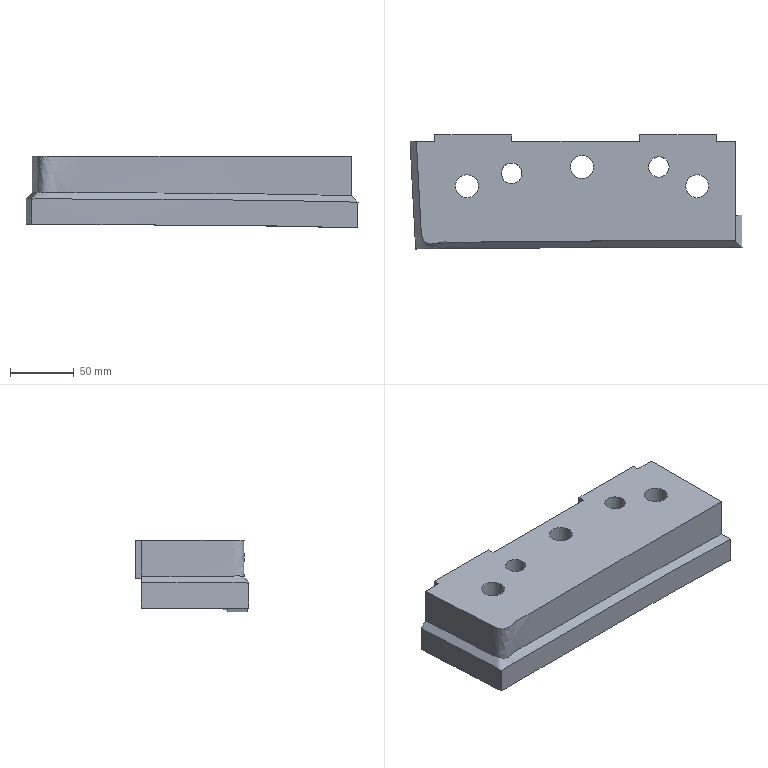Part | NX | features solid 2 | 1 solid | 38 faces | box 259.399 x 88.994 x 55.9 mm | volume 789888 mm3 | plane 20 | cylinder 10 | spline 6 | cone 2 | commonest cylinder face diameters 18 x3 26 x3 16 x2 36 x2